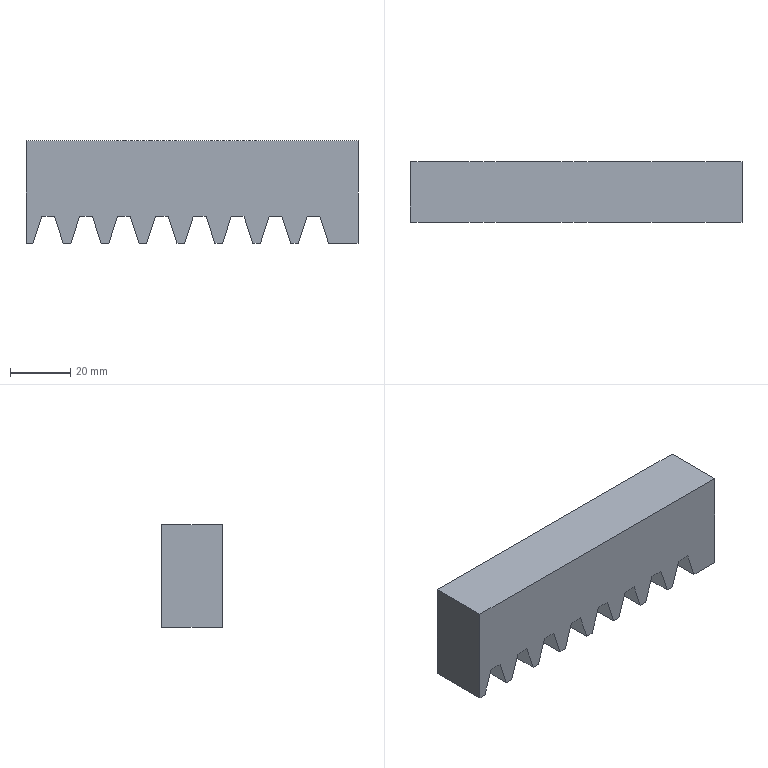Part | SolidWorks | features BaseBody 1 | 1 solid | 46 faces | box 110 x 20 x 34 mm | volume 64536 mm3 | plane 30 | cylinder 16 | commonest cylinder face diameters 94.224 x16
STEP:
#1=CARTESIAN_POINT('',(107.487,369.5,-21.002));
#2=VERTEX_POINT('',#1);
#3=CARTESIAN_POINT('',(109.612,369.5,-21.05));
#4=VERTEX_POINT('',#3);
#5=CARTESIAN_POINT('',(107.487,369.5,-68.114));
#6=DIRECTION('',(0.,1.,0.));
#7=DIRECTION('',(0.,0.,1.));
#8=AXIS2_PLACEMENT_3D('',#5,#6,#7);
#9=CIRCLE('',#8,47.112);
#10=EDGE_CURVE('',#2,#4,#9,.T.);
#11=ORIENTED_EDGE('',*,*,#10,.F.);
#12=CARTESIAN_POINT('',(107.487,389.5,-21.002));
#13=VERTEX_POINT('',#12);
#14=CARTESIAN_POINT('',(107.487,379.5,-21.002));
#15=DIRECTION('',(0.,1.,0.));
#16=VECTOR('',#15,1000.);
#17=LINE('',#14,#16);
#18=EDGE_CURVE('',#2,#13,#17,.T.);
#19=ORIENTED_EDGE('',*,*,#18,.T.);
#20=CARTESIAN_POINT('',(109.612,389.5,-21.05));
#21=VERTEX_POINT('',#20);
#22=CARTESIAN_POINT('',(107.487,389.5,-68.114));
#23=DIRECTION('',(0.,-1.,0.));
#24=DIRECTION('',(0.,0.,1.));
#25=AXIS2_PLACEMENT_3D('',#22,#23,#24);
#26=CIRCLE('',#25,47.112);
#27=EDGE_CURVE('',#21,#13,#26,.T.);
#28=ORIENTED_EDGE('',*,*,#27,.F.);
#29=CARTESIAN_POINT('',(109.612,369.5,-21.05));
#30=DIRECTION('',(0.,1.,0.));
#31=VECTOR('',#30,1000.);
#32=LINE('',#29,#31);
#33=EDGE_CURVE('',#4,#21,#32,.T.);
#34=ORIENTED_EDGE('',*,*,#33,.F.);
#35=EDGE_LOOP('',(#11,#19,#28,#34));
#36=FACE_OUTER_BOUND('',#35,.T.);
#37=CARTESIAN_POINT('',(107.487,379.5,-68.114));
#38=DIRECTION('',(0.,1.,0.));
#39=DIRECTION('',(0.,0.,1.));
#40=AXIS2_PLACEMENT_3D('',#37,#38,#39);
#41=CYLINDRICAL_SURFACE('',#40,47.112);
#42=ADVANCED_FACE('',(#36),#41,.F.);
#43=CARTESIAN_POINT('',(94.927,369.5,-21.002));
#44=VERTEX_POINT('',#43);
#45=CARTESIAN_POINT('',(97.052,369.5,-21.05));
#46=VERTEX_POINT('',#45);
#47=CARTESIAN_POINT('',(94.927,369.5,-68.114));
#48=DIRECTION('',(0.,1.,0.));
#49=DIRECTION('',(0.,0.,1.));
#50=AXIS2_PLACEMENT_3D('',#47,#48,#49);
#51=CIRCLE('',#50,47.112);
#52=EDGE_CURVE('',#44,#46,#51,.T.);
#53=ORIENTED_EDGE('',*,*,#52,.F.);
#54=CARTESIAN_POINT('',(94.927,389.5,-21.002));
#55=VERTEX_POINT('',#54);
#56=CARTESIAN_POINT('',(94.927,379.5,-21.002));
#57=DIRECTION('',(0.,1.,0.));
#58=VECTOR('',#57,1000.);
#59=LINE('',#56,#58);
#60=EDGE_CURVE('',#44,#55,#59,.T.);
#61=ORIENTED_EDGE('',*,*,#60,.T.);
#62=CARTESIAN_POINT('',(97.052,389.5,-21.05));
#63=VERTEX_POINT('',#62);
#64=CARTESIAN_POINT('',(94.927,389.5,-68.114));
#65=DIRECTION('',(0.,-1.,0.));
#66=DIRECTION('',(0.,0.,1.));
#67=AXIS2_PLACEMENT_3D('',#64,#65,#66);
#68=CIRCLE('',#67,47.112);
#69=EDGE_CURVE('',#63,#55,#68,.T.);
#70=ORIENTED_EDGE('',*,*,#69,.F.);
#71=CARTESIAN_POINT('',(97.052,369.5,-21.05));
#72=DIRECTION('',(0.,1.,0.));
#73=VECTOR('',#72,1000.);
#74=LINE('',#71,#73);
#75=EDGE_CURVE('',#46,#63,#74,.T.);
#76=ORIENTED_EDGE('',*,*,#75,.F.);
#77=EDGE_LOOP('',(#53,#61,#70,#76));
#78=FACE_OUTER_BOUND('',#77,.T.);
#79=CARTESIAN_POINT('',(94.927,379.5,-68.114));
#80=DIRECTION('',(0.,1.,0.));
#81=DIRECTION('',(0.,0.,1.));
#82=AXIS2_PLACEMENT_3D('',#79,#80,#81);
#83=CYLINDRICAL_SURFACE('',#82,47.112);
#84=ADVANCED_FACE('',(#78),#83,.F.);
#85=CARTESIAN_POINT('',(82.367,369.5,-21.002));
#86=VERTEX_POINT('',#85);
#87=CARTESIAN_POINT('',(84.492,369.5,-21.05));
#88=VERTEX_POINT('',#87);
#89=CARTESIAN_POINT('',(82.367,369.5,-68.114));
#90=DIRECTION('',(0.,1.,0.));
#91=DIRECTION('',(0.,0.,1.));
#92=AXIS2_PLACEMENT_3D('',#89,#90,#91);
#93=CIRCLE('',#92,47.112);
#94=EDGE_CURVE('',#86,#88,#93,.T.);
#95=ORIENTED_EDGE('',*,*,#94,.F.);
#96=CARTESIAN_POINT('',(82.367,389.5,-21.002));
#97=VERTEX_POINT('',#96);
#98=CARTESIAN_POINT('',(82.367,379.5,-21.002));
#99=DIRECTION('',(0.,1.,0.));
#100=VECTOR('',#99,1000.);
#101=LINE('',#98,#100);
#102=EDGE_CURVE('',#86,#97,#101,.T.);
#103=ORIENTED_EDGE('',*,*,#102,.T.);
#104=CARTESIAN_POINT('',(84.492,389.5,-21.05));
#105=VERTEX_POINT('',#104);
#106=CARTESIAN_POINT('',(82.367,389.5,-68.114));
#107=DIRECTION('',(0.,-1.,0.));
#108=DIRECTION('',(0.,0.,1.));
#109=AXIS2_PLACEMENT_3D('',#106,#107,#108);
#110=CIRCLE('',#109,47.112);
#111=EDGE_CURVE('',#105,#97,#110,.T.);
#112=ORIENTED_EDGE('',*,*,#111,.F.);
#113=CARTESIAN_POINT('',(84.492,369.5,-21.05));
#114=DIRECTION('',(0.,1.,0.));
#115=VECTOR('',#114,1000.);
#116=LINE('',#113,#115);
#117=EDGE_CURVE('',#88,#105,#116,.T.);
#118=ORIENTED_EDGE('',*,*,#117,.F.);
#119=EDGE_LOOP('',(#95,#103,#112,#118));
#120=FACE_OUTER_BOUND('',#119,.T.);
#121=CARTESIAN_POINT('',(82.367,379.5,-68.114));
#122=DIRECTION('',(0.,1.,0.));
#123=DIRECTION('',(0.,0.,1.));
#124=AXIS2_PLACEMENT_3D('',#121,#122,#123);
#125=CYLINDRICAL_SURFACE('',#124,47.112);
#126=ADVANCED_FACE('',(#120),#125,.F.);
#127=CARTESIAN_POINT('',(69.807,369.5,-21.002));
#128=VERTEX_POINT('',#127);
#129=CARTESIAN_POINT('',(71.932,369.5,-21.05));
#130=VERTEX_POINT('',#129);
#131=CARTESIAN_POINT('',(69.807,369.5,-68.114));
#132=DIRECTION('',(0.,1.,0.));
#133=DIRECTION('',(0.,0.,1.));
#134=AXIS2_PLACEMENT_3D('',#131,#132,#133);
#135=CIRCLE('',#134,47.112);
#136=EDGE_CURVE('',#128,#130,#135,.T.);
#137=ORIENTED_EDGE('',*,*,#136,.F.);
#138=CARTESIAN_POINT('',(69.807,389.5,-21.002));
#139=VERTEX_POINT('',#138);
#140=CARTESIAN_POINT('',(69.807,379.5,-21.002));
#141=DIRECTION('',(0.,1.,0.));
#142=VECTOR('',#141,1000.);
#143=LINE('',#140,#142);
#144=EDGE_CURVE('',#128,#139,#143,.T.);
#145=ORIENTED_EDGE('',*,*,#144,.T.);
#146=CARTESIAN_POINT('',(71.932,389.5,-21.05));
#147=VERTEX_POINT('',#146);
#148=CARTESIAN_POINT('',(69.807,389.5,-68.114));
#149=DIRECTION('',(0.,-1.,0.));
#150=DIRECTION('',(0.,0.,1.));
#151=AXIS2_PLACEMENT_3D('',#148,#149,#150);
#152=CIRCLE('',#151,47.112);
#153=EDGE_CURVE('',#147,#139,#152,.T.);
#154=ORIENTED_EDGE('',*,*,#153,.F.);
#155=CARTESIAN_POINT('',(71.932,369.5,-21.05));
#156=DIRECTION('',(0.,1.,0.));
#157=VECTOR('',#156,1000.);
#158=LINE('',#155,#157);
#159=EDGE_CURVE('',#130,#147,#158,.T.);
#160=ORIENTED_EDGE('',*,*,#159,.F.);
#161=EDGE_LOOP('',(#137,#145,#154,#160));
#162=FACE_OUTER_BOUND('',#161,.T.);
#163=CARTESIAN_POINT('',(69.807,379.5,-68.114));
#164=DIRECTION('',(0.,1.,0.));
#165=DIRECTION('',(0.,0.,1.));
#166=AXIS2_PLACEMENT_3D('',#163,#164,#165);
#167=CYLINDRICAL_SURFACE('',#166,47.112);
#168=ADVANCED_FACE('',(#162),#167,.F.);
#169=CARTESIAN_POINT('',(57.247,369.5,-21.002));
#170=VERTEX_POINT('',#169);
#171=CARTESIAN_POINT('',(59.372,369.5,-21.05));
#172=VERTEX_POINT('',#171);
#173=CARTESIAN_POINT('',(57.247,369.5,-68.114));
#174=DIRECTION('',(0.,1.,0.));
#175=DIRECTION('',(0.,0.,1.));
#176=AXIS2_PLACEMENT_3D('',#173,#174,#175);
#177=CIRCLE('',#176,47.112);
#178=EDGE_CURVE('',#170,#172,#177,.T.);
#179=ORIENTED_EDGE('',*,*,#178,.F.);
#180=CARTESIAN_POINT('',(57.247,389.5,-21.002));
#181=VERTEX_POINT('',#180);
#182=CARTESIAN_POINT('',(57.247,379.5,-21.002));
#183=DIRECTION('',(0.,1.,0.));
#184=VECTOR('',#183,1000.);
#185=LINE('',#182,#184);
#186=EDGE_CURVE('',#170,#181,#185,.T.);
#187=ORIENTED_EDGE('',*,*,#186,.T.);
#188=CARTESIAN_POINT('',(59.372,389.5,-21.05));
#189=VERTEX_POINT('',#188);
#190=CARTESIAN_POINT('',(57.247,389.5,-68.114));
#191=DIRECTION('',(0.,-1.,0.));
#192=DIRECTION('',(0.,0.,1.));
#193=AXIS2_PLACEMENT_3D('',#190,#191,#192);
#194=CIRCLE('',#193,47.112);
#195=EDGE_CURVE('',#189,#181,#194,.T.);
#196=ORIENTED_EDGE('',*,*,#195,.F.);
#197=CARTESIAN_POINT('',(59.372,369.5,-21.05));
#198=DIRECTION('',(0.,1.,0.));
#199=VECTOR('',#198,1000.);
#200=LINE('',#197,#199);
#201=EDGE_CURVE('',#172,#189,#200,.T.);
#202=ORIENTED_EDGE('',*,*,#201,.F.);
#203=EDGE_LOOP('',(#179,#187,#196,#202));
#204=FACE_OUTER_BOUND('',#203,.T.);
#205=CARTESIAN_POINT('',(57.247,379.5,-68.114));
#206=DIRECTION('',(0.,1.,0.));
#207=DIRECTION('',(0.,0.,1.));
#208=AXIS2_PLACEMENT_3D('',#205,#206,#207);
#209=CYLINDRICAL_SURFACE('',#208,47.112);
#210=ADVANCED_FACE('',(#204),#209,.F.);
#211=CARTESIAN_POINT('',(44.687,369.5,-21.002));
#212=VERTEX_POINT('',#211);
#213=CARTESIAN_POINT('',(46.812,369.5,-21.05));
#214=VERTEX_POINT('',#213);
#215=CARTESIAN_POINT('',(44.687,369.5,-68.114));
#216=DIRECTION('',(0.,1.,0.));
#217=DIRECTION('',(0.,0.,1.));
#218=AXIS2_PLACEMENT_3D('',#215,#216,#217);
#219=CIRCLE('',#218,47.112);
#220=EDGE_CURVE('',#212,#214,#219,.T.);
#221=ORIENTED_EDGE('',*,*,#220,.F.);
#222=CARTESIAN_POINT('',(44.687,389.5,-21.002));
#223=VERTEX_POINT('',#222);
#224=CARTESIAN_POINT('',(44.687,379.5,-21.002));
#225=DIRECTION('',(0.,1.,0.));
#226=VECTOR('',#225,1000.);
#227=LINE('',#224,#226);
#228=EDGE_CURVE('',#212,#223,#227,.T.);
#229=ORIENTED_EDGE('',*,*,#228,.T.);
#230=CARTESIAN_POINT('',(46.812,389.5,-21.05));
#231=VERTEX_POINT('',#230);
#232=CARTESIAN_POINT('',(44.687,389.5,-68.114));
#233=DIRECTION('',(0.,-1.,0.));
#234=DIRECTION('',(0.,0.,1.));
#235=AXIS2_PLACEMENT_3D('',#232,#233,#234);
#236=CIRCLE('',#235,47.112);
#237=EDGE_CURVE('',#231,#223,#236,.T.);
#238=ORIENTED_EDGE('',*,*,#237,.F.);
#239=CARTESIAN_POINT('',(46.812,369.5,-21.05));
#240=DIRECTION('',(0.,1.,0.));
#241=VECTOR('',#240,1000.);
#242=LINE('',#239,#241);
#243=EDGE_CURVE('',#214,#231,#242,.T.);
#244=ORIENTED_EDGE('',*,*,#243,.F.);
#245=EDGE_LOOP('',(#221,#229,#238,#244));
#246=FACE_OUTER_BOUND('',#245,.T.);
#247=CARTESIAN_POINT('',(44.687,379.5,-68.114));
#248=DIRECTION('',(0.,1.,0.));
#249=DIRECTION('',(0.,0.,1.));
#250=AXIS2_PLACEMENT_3D('',#247,#248,#249);
#251=CYLINDRICAL_SURFACE('',#250,47.112);
#252=ADVANCED_FACE('',(#246),#251,.F.);
#253=CARTESIAN_POINT('',(32.127,369.5,-21.002));
#254=VERTEX_POINT('',#253);
#255=CARTESIAN_POINT('',(34.252,369.5,-21.05));
#256=VERTEX_POINT('',#255);
#257=CARTESIAN_POINT('',(32.127,369.5,-68.114));
#258=DIRECTION('',(0.,1.,0.));
#259=DIRECTION('',(0.,0.,1.));
#260=AXIS2_PLACEMENT_3D('',#257,#258,#259);
#261=CIRCLE('',#260,47.112);
#262=EDGE_CURVE('',#254,#256,#261,.T.);
#263=ORIENTED_EDGE('',*,*,#262,.F.);
#264=CARTESIAN_POINT('',(32.127,389.5,-21.002));
#265=VERTEX_POINT('',#264);
#266=CARTESIAN_POINT('',(32.127,379.5,-21.002));
#267=DIRECTION('',(0.,1.,0.));
#268=VECTOR('',#267,1000.);
#269=LINE('',#266,#268);
#270=EDGE_CURVE('',#254,#265,#269,.T.);
#271=ORIENTED_EDGE('',*,*,#270,.T.);
#272=CARTESIAN_POINT('',(34.252,389.5,-21.05));
#273=VERTEX_POINT('',#272);
#274=CARTESIAN_POINT('',(32.127,389.5,-68.114));
#275=DIRECTION('',(0.,-1.,0.));
#276=DIRECTION('',(0.,0.,1.));
#277=AXIS2_PLACEMENT_3D('',#274,#275,#276);
#278=CIRCLE('',#277,47.112);
#279=EDGE_CURVE('',#273,#265,#278,.T.);
#280=ORIENTED_EDGE('',*,*,#279,.F.);
#281=CARTESIAN_POINT('',(34.252,369.5,-21.05));
#282=DIRECTION('',(0.,1.,0.));
#283=VECTOR('',#282,1000.);
#284=LINE('',#281,#283);
#285=EDGE_CURVE('',#256,#273,#284,.T.);
#286=ORIENTED_EDGE('',*,*,#285,.F.);
#287=EDGE_LOOP('',(#263,#271,#280,#286));
#288=FACE_OUTER_BOUND('',#287,.T.);
#289=CARTESIAN_POINT('',(32.127,379.5,-68.114));
#290=DIRECTION('',(0.,1.,0.));
#291=DIRECTION('',(0.,0.,1.));
#292=AXIS2_PLACEMENT_3D('',#289,#290,#291);
#293=CYLINDRICAL_SURFACE('',#292,47.112);
#294=ADVANCED_FACE('',(#288),#293,.F.);
#295=CARTESIAN_POINT('',(19.567,369.5,-21.002));
#296=VERTEX_POINT('',#295);
#297=CARTESIAN_POINT('',(21.692,369.5,-21.05));
#298=VERTEX_POINT('',#297);
#299=CARTESIAN_POINT('',(19.567,369.5,-68.114));
#300=DIRECTION('',(0.,1.,0.));
#301=DIRECTION('',(0.,0.,1.));
#302=AXIS2_PLACEMENT_3D('',#299,#300,#301);
#303=CIRCLE('',#302,47.112);
#304=EDGE_CURVE('',#296,#298,#303,.T.);
#305=ORIENTED_EDGE('',*,*,#304,.F.);
#306=CARTESIAN_POINT('',(19.567,389.5,-21.002));
#307=VERTEX_POINT('',#306);
#308=CARTESIAN_POINT('',(19.567,379.5,-21.002));
#309=DIRECTION('',(0.,1.,0.));
#310=VECTOR('',#309,1000.);
#311=LINE('',#308,#310);
#312=EDGE_CURVE('',#296,#307,#311,.T.);
#313=ORIENTED_EDGE('',*,*,#312,.T.);
#314=CARTESIAN_POINT('',(21.692,389.5,-21.05));
#315=VERTEX_POINT('',#314);
#316=CARTESIAN_POINT('',(19.567,389.5,-68.114));
#317=DIRECTION('',(0.,-1.,0.));
#318=DIRECTION('',(0.,0.,1.));
#319=AXIS2_PLACEMENT_3D('',#316,#317,#318);
#320=CIRCLE('',#319,47.112);
#321=EDGE_CURVE('',#315,#307,#320,.T.);
#322=ORIENTED_EDGE('',*,*,#321,.F.);
#323=CARTESIAN_POINT('',(21.692,369.5,-21.05));
#324=DIRECTION('',(0.,1.,0.));
#325=VECTOR('',#324,1000.);
#326=LINE('',#323,#325);
#327=EDGE_CURVE('',#298,#315,#326,.T.);
#328=ORIENTED_EDGE('',*,*,#327,.F.);
#329=EDGE_LOOP('',(#305,#313,#322,#328));
#330=FACE_OUTER_BOUND('',#329,.T.);
#331=CARTESIAN_POINT('',(19.567,379.5,-68.114));
#332=DIRECTION('',(0.,1.,0.));
#333=DIRECTION('',(0.,0.,1.));
#334=AXIS2_PLACEMENT_3D('',#331,#332,#333);
#335=CYLINDRICAL_SURFACE('',#334,47.112);
#336=ADVANCED_FACE('',(#330),#335,.F.);
#337=CARTESIAN_POINT('',(112.513,369.5,-30.));
#338=VERTEX_POINT('',#337);
#339=CARTESIAN_POINT('',(109.612,369.5,-21.05));
#340=DIRECTION('',(0.3083,0.,-0.9513));
#341=VECTOR('',#340,1000.);
#342=LINE('',#339,#341);
#343=EDGE_CURVE('',#4,#338,#342,.T.);
#344=ORIENTED_EDGE('',*,*,#343,.T.);
#345=CARTESIAN_POINT('',(122.247,369.5,-30.));
#346=VERTEX_POINT('',#345);
#347=CARTESIAN_POINT('',(77.247,369.5,-30.));
#348=DIRECTION('',(1.,0.,0.));
#349=VECTOR('',#348,1000.);
#350=LINE('',#347,#349);
#351=EDGE_CURVE('',#338,#346,#350,.T.);
#352=ORIENTED_EDGE('',*,*,#351,.T.);
#353=CARTESIAN_POINT('',(122.247,369.5,4.));
#354=VERTEX_POINT('',#353);
#355=CARTESIAN_POINT('',(122.247,369.5,-76.043));
#356=DIRECTION('',(0.,0.,1.));
#357=VECTOR('',#356,1000.);
#358=LINE('',#355,#357);
#359=EDGE_CURVE('',#346,#354,#358,.T.);
#360=ORIENTED_EDGE('',*,*,#359,.T.);
#361=CARTESIAN_POINT('',(12.247,369.5,4.));
#362=VERTEX_POINT('',#361);
#363=CARTESIAN_POINT('',(77.247,369.5,4.));
#364=DIRECTION('',(-1.,0.,0.));
#365=VECTOR('',#364,1000.);
#366=LINE('',#363,#365);
#367=EDGE_CURVE('',#354,#362,#366,.T.);
#368=ORIENTED_EDGE('',*,*,#367,.T.);
#369=CARTESIAN_POINT('',(12.247,369.5,-30.));
#370=VERTEX_POINT('',#369);
#371=CARTESIAN_POINT('',(12.247,369.5,-76.043));
#372=DIRECTION('',(0.,0.,-1.));
#373=VECTOR('',#372,1000.);
#374=LINE('',#371,#373);
#375=EDGE_CURVE('',#362,#370,#374,.T.);
#376=ORIENTED_EDGE('',*,*,#375,.T.);
#377=CARTESIAN_POINT('',(14.54,369.5,-30.));
#378=VERTEX_POINT('',#377);
#379=CARTESIAN_POINT('',(77.247,369.5,-30.));
#380=DIRECTION('',(1.,0.,0.));
#381=VECTOR('',#380,1000.);
#382=LINE('',#379,#381);
#383=EDGE_CURVE('',#370,#378,#382,.T.);
#384=ORIENTED_EDGE('',*,*,#383,.T.);
#385=CARTESIAN_POINT('',(17.441,369.5,-21.05));
#386=VERTEX_POINT('',#385);
#387=CARTESIAN_POINT('',(14.54,369.5,-30.));
#388=DIRECTION('',(0.3083,0.,0.9513));
#389=VECTOR('',#388,1000.);
#390=LINE('',#387,#389);
#391=EDGE_CURVE('',#378,#386,#390,.T.);
#392=ORIENTED_EDGE('',*,*,#391,.T.);
#393=CARTESIAN_POINT('',(19.567,369.5,-68.114));
#394=DIRECTION('',(0.,1.,0.));
#395=DIRECTION('',(0.,0.,1.));
#396=AXIS2_PLACEMENT_3D('',#393,#394,#395);
#397=CIRCLE('',#396,47.112);
#398=EDGE_CURVE('',#386,#296,#397,.T.);
#399=ORIENTED_EDGE('',*,*,#398,.T.);
#400=ORIENTED_EDGE('',*,*,#304,.T.);
#401=CARTESIAN_POINT('',(24.593,369.5,-30.));
#402=VERTEX_POINT('',#401);
#403=CARTESIAN_POINT('',(43.101,369.5,-87.109));
#404=DIRECTION('',(0.3083,0.,-0.9513));
#405=VECTOR('',#404,1000.);
#406=LINE('',#403,#405);
#407=EDGE_CURVE('',#298,#402,#406,.T.);
#408=ORIENTED_EDGE('',*,*,#407,.T.);
#409=CARTESIAN_POINT('',(27.1,369.5,-30.));
#410=VERTEX_POINT('',#409);
#411=CARTESIAN_POINT('',(77.247,369.5,-30.));
#412=DIRECTION('',(1.,0.,0.));
#413=VECTOR('',#412,1000.);
#414=LINE('',#411,#413);
#415=EDGE_CURVE('',#402,#410,#414,.T.);
#416=ORIENTED_EDGE('',*,*,#415,.T.);
#417=CARTESIAN_POINT('',(30.001,369.5,-21.05));
#418=VERTEX_POINT('',#417);
#419=CARTESIAN_POINT('',(27.1,369.5,-30.));
#420=DIRECTION('',(0.3083,0.,0.9513));
#421=VECTOR('',#420,1000.);
#422=LINE('',#419,#421);
#423=EDGE_CURVE('',#410,#418,#422,.T.);
#424=ORIENTED_EDGE('',*,*,#423,.T.);
#425=CARTESIAN_POINT('',(32.127,369.5,-68.114));
#426=DIRECTION('',(0.,1.,0.));
#427=DIRECTION('',(0.,0.,1.));
#428=AXIS2_PLACEMENT_3D('',#425,#426,#427);
#429=CIRCLE('',#428,47.112);
#430=EDGE_CURVE('',#418,#254,#429,.T.);
#431=ORIENTED_EDGE('',*,*,#430,.T.);
#432=ORIENTED_EDGE('',*,*,#262,.T.);
#433=CARTESIAN_POINT('',(37.153,369.5,-30.));
#434=VERTEX_POINT('',#433);
#435=CARTESIAN_POINT('',(34.252,369.5,-21.05));
#436=DIRECTION('',(0.3083,0.,-0.9513));
#437=VECTOR('',#436,1000.);
#438=LINE('',#435,#437);
#439=EDGE_CURVE('',#256,#434,#438,.T.);
#440=ORIENTED_EDGE('',*,*,#439,.T.);
#441=CARTESIAN_POINT('',(39.66,369.5,-30.));
#442=VERTEX_POINT('',#441);
#443=CARTESIAN_POINT('',(77.247,369.5,-30.));
#444=DIRECTION('',(1.,0.,0.));
#445=VECTOR('',#444,1000.);
#446=LINE('',#443,#445);
#447=EDGE_CURVE('',#434,#442,#446,.T.);
#448=ORIENTED_EDGE('',*,*,#447,.T.);
#449=CARTESIAN_POINT('',(42.561,369.5,-21.05));
#450=VERTEX_POINT('',#449);
#451=CARTESIAN_POINT('',(39.66,369.5,-30.));
#452=DIRECTION('',(0.3083,0.,0.9513));
#453=VECTOR('',#452,1000.);
#454=LINE('',#451,#453);
#455=EDGE_CURVE('',#442,#450,#454,.T.);
#456=ORIENTED_EDGE('',*,*,#455,.T.);
#457=CARTESIAN_POINT('',(44.687,369.5,-68.114));
#458=DIRECTION('',(0.,1.,0.));
#459=DIRECTION('',(0.,0.,1.));
#460=AXIS2_PLACEMENT_3D('',#457,#458,#459);
#461=CIRCLE('',#460,47.112);
#462=EDGE_CURVE('',#450,#212,#461,.T.);
#463=ORIENTED_EDGE('',*,*,#462,.T.);
#464=ORIENTED_EDGE('',*,*,#220,.T.);
#465=CARTESIAN_POINT('',(49.713,369.5,-30.));
#466=VERTEX_POINT('',#465);
#467=CARTESIAN_POINT('',(46.812,369.5,-21.05));
#468=DIRECTION('',(0.3083,0.,-0.9513));
#469=VECTOR('',#468,1000.);
#470=LINE('',#467,#469);
#471=EDGE_CURVE('',#214,#466,#470,.T.);
#472=ORIENTED_EDGE('',*,*,#471,.T.);
#473=CARTESIAN_POINT('',(52.22,369.5,-30.));
#474=VERTEX_POINT('',#473);
#475=CARTESIAN_POINT('',(77.247,369.5,-30.));
#476=DIRECTION('',(1.,0.,0.));
#477=VECTOR('',#476,1000.);
#478=LINE('',#475,#477);
#479=EDGE_CURVE('',#466,#474,#478,.T.);
#480=ORIENTED_EDGE('',*,*,#479,.T.);
#481=CARTESIAN_POINT('',(55.121,369.5,-21.05));
#482=VERTEX_POINT('',#481);
#483=CARTESIAN_POINT('',(52.22,369.5,-30.));
#484=DIRECTION('',(0.3083,0.,0.9513));
#485=VECTOR('',#484,1000.);
#486=LINE('',#483,#485);
#487=EDGE_CURVE('',#474,#482,#486,.T.);
#488=ORIENTED_EDGE('',*,*,#487,.T.);
#489=CARTESIAN_POINT('',(57.247,369.5,-68.114));
#490=DIRECTION('',(0.,1.,0.));
#491=DIRECTION('',(0.,0.,1.));
#492=AXIS2_PLACEMENT_3D('',#489,#490,#491);
#493=CIRCLE('',#492,47.112);
#494=EDGE_CURVE('',#482,#170,#493,.T.);
#495=ORIENTED_EDGE('',*,*,#494,.T.);
#496=ORIENTED_EDGE('',*,*,#178,.T.);
#497=CARTESIAN_POINT('',(62.273,369.5,-30.));
#498=VERTEX_POINT('',#497);
#499=CARTESIAN_POINT('',(59.372,369.5,-21.05));
#500=DIRECTION('',(0.3083,0.,-0.9513));
#501=VECTOR('',#500,1000.);
#502=LINE('',#499,#501);
#503=EDGE_CURVE('',#172,#498,#502,.T.);
#504=ORIENTED_EDGE('',*,*,#503,.T.);
#505=CARTESIAN_POINT('',(64.78,369.5,-30.));
#506=VERTEX_POINT('',#505);
#507=CARTESIAN_POINT('',(77.247,369.5,-30.));
#508=DIRECTION('',(1.,0.,0.));
#509=VECTOR('',#508,1000.);
#510=LINE('',#507,#509);
#511=EDGE_CURVE('',#498,#506,#510,.T.);
#512=ORIENTED_EDGE('',*,*,#511,.T.);
#513=CARTESIAN_POINT('',(67.681,369.5,-21.05));
#514=VERTEX_POINT('',#513);
#515=CARTESIAN_POINT('',(64.78,369.5,-30.));
#516=DIRECTION('',(0.3083,0.,0.9513));
#517=VECTOR('',#516,1000.);
#518=LINE('',#515,#517);
#519=EDGE_CURVE('',#506,#514,#518,.T.);
#520=ORIENTED_EDGE('',*,*,#519,.T.);
#521=CARTESIAN_POINT('',(69.807,369.5,-68.114));
#522=DIRECTION('',(0.,1.,0.));
#523=DIRECTION('',(0.,0.,1.));
#524=AXIS2_PLACEMENT_3D('',#521,#522,#523);
#525=CIRCLE('',#524,47.112);
#526=EDGE_CURVE('',#514,#128,#525,.T.);
#527=ORIENTED_EDGE('',*,*,#526,.T.);
#528=ORIENTED_EDGE('',*,*,#136,.T.);
#529=CARTESIAN_POINT('',(74.833,369.5,-30.));
#530=VERTEX_POINT('',#529);
#531=CARTESIAN_POINT('',(71.932,369.5,-21.05));
#532=DIRECTION('',(0.3083,0.,-0.9513));
#533=VECTOR('',#532,1000.);
#534=LINE('',#531,#533);
#535=EDGE_CURVE('',#130,#530,#534,.T.);
#536=ORIENTED_EDGE('',*,*,#535,.T.);
#537=CARTESIAN_POINT('',(77.34,369.5,-30.));
#538=VERTEX_POINT('',#537);
#539=CARTESIAN_POINT('',(77.247,369.5,-30.));
#540=DIRECTION('',(1.,0.,0.));
#541=VECTOR('',#540,1000.);
#542=LINE('',#539,#541);
#543=EDGE_CURVE('',#530,#538,#542,.T.);
#544=ORIENTED_EDGE('',*,*,#543,.T.);
#545=CARTESIAN_POINT('',(80.241,369.5,-21.05));
#546=VERTEX_POINT('',#545);
#547=CARTESIAN_POINT('',(77.34,369.5,-30.));
#548=DIRECTION('',(0.3083,0.,0.9513));
#549=VECTOR('',#548,1000.);
#550=LINE('',#547,#549);
#551=EDGE_CURVE('',#538,#546,#550,.T.);
#552=ORIENTED_EDGE('',*,*,#551,.T.);
#553=CARTESIAN_POINT('',(82.367,369.5,-68.114));
#554=DIRECTION('',(0.,1.,0.));
#555=DIRECTION('',(0.,0.,1.));
#556=AXIS2_PLACEMENT_3D('',#553,#554,#555);
#557=CIRCLE('',#556,47.112);
#558=EDGE_CURVE('',#546,#86,#557,.T.);
#559=ORIENTED_EDGE('',*,*,#558,.T.);
#560=ORIENTED_EDGE('',*,*,#94,.T.);
#561=CARTESIAN_POINT('',(87.393,369.5,-30.));
#562=VERTEX_POINT('',#561);
#563=CARTESIAN_POINT('',(84.492,369.5,-21.05));
#564=DIRECTION('',(0.3083,0.,-0.9513));
#565=VECTOR('',#564,1000.);
#566=LINE('',#563,#565);
#567=EDGE_CURVE('',#88,#562,#566,.T.);
#568=ORIENTED_EDGE('',*,*,#567,.T.);
#569=CARTESIAN_POINT('',(89.9,369.5,-30.));
#570=VERTEX_POINT('',#569);
#571=CARTESIAN_POINT('',(77.247,369.5,-30.));
#572=DIRECTION('',(1.,0.,0.));
#573=VECTOR('',#572,1000.);
#574=LINE('',#571,#573);
#575=EDGE_CURVE('',#562,#570,#574,.T.);
#576=ORIENTED_EDGE('',*,*,#575,.T.);
#577=CARTESIAN_POINT('',(92.801,369.5,-21.05));
#578=VERTEX_POINT('',#577);
#579=CARTESIAN_POINT('',(89.9,369.5,-30.));
#580=DIRECTION('',(0.3083,0.,0.9513));
#581=VECTOR('',#580,1000.);
#582=LINE('',#579,#581);
#583=EDGE_CURVE('',#570,#578,#582,.T.);
#584=ORIENTED_EDGE('',*,*,#583,.T.);
#585=CARTESIAN_POINT('',(94.927,369.5,-68.114));
#586=DIRECTION('',(0.,1.,0.));
#587=DIRECTION('',(0.,0.,1.));
#588=AXIS2_PLACEMENT_3D('',#585,#586,#587);
#589=CIRCLE('',#588,47.112);
#590=EDGE_CURVE('',#578,#44,#589,.T.);
#591=ORIENTED_EDGE('',*,*,#590,.T.);
#592=ORIENTED_EDGE('',*,*,#52,.T.);
#593=CARTESIAN_POINT('',(99.953,369.5,-30.));
#594=VERTEX_POINT('',#593);
#595=CARTESIAN_POINT('',(97.052,369.5,-21.05));
#596=DIRECTION('',(0.3083,0.,-0.9513));
#597=VECTOR('',#596,1000.);
#598=LINE('',#595,#597);
#599=EDGE_CURVE('',#46,#594,#598,.T.);
#600=ORIENTED_EDGE('',*,*,#599,.T.);
#601=CARTESIAN_POINT('',(102.46,369.5,-30.));
#602=VERTEX_POINT('',#601);
#603=CARTESIAN_POINT('',(77.247,369.5,-30.));
#604=DIRECTION('',(1.,0.,0.));
#605=VECTOR('',#604,1000.);
#606=LINE('',#603,#605);
#607=EDGE_CURVE('',#594,#602,#606,.T.);
#608=ORIENTED_EDGE('',*,*,#607,.T.);
#609=CARTESIAN_POINT('',(105.361,369.5,-21.05));
#610=VERTEX_POINT('',#609);
#611=CARTESIAN_POINT('',(102.46,369.5,-30.));
#612=DIRECTION('',(0.3083,0.,0.9513));
#613=VECTOR('',#612,1000.);
#614=LINE('',#611,#613);
#615=EDGE_CURVE('',#602,#610,#614,.T.);
#616=ORIENTED_EDGE('',*,*,#615,.T.);
#617=CARTESIAN_POINT('',(107.487,369.5,-68.114));
#618=DIRECTION('',(0.,1.,0.));
#619=DIRECTION('',(0.,0.,1.));
#620=AXIS2_PLACEMENT_3D('',#617,#618,#619);
#621=CIRCLE('',#620,47.112);
#622=EDGE_CURVE('',#610,#2,#621,.T.);
#623=ORIENTED_EDGE('',*,*,#622,.T.);
#624=ORIENTED_EDGE('',*,*,#10,.T.);
#625=EDGE_LOOP('',(#344,#352,#360,#368,#376,#384,#392,#399,#400,#408,#416,#424,#431,#432,#440,#448,#456,#463,#464,#472,#480,#488,#495,#496,#504,#512,#520,#527,#528,#536,#544,#552,#559,#560,#568,#576,#584,#591,#592,#600,#608,#616,#623,#624));
#626=FACE_OUTER_BOUND('',#625,.T.);
#627=CARTESIAN_POINT('',(77.247,369.5,-76.043));
#628=DIRECTION('',(0.,-1.,0.));
#629=DIRECTION('',(0.,0.,-1.));
#630=AXIS2_PLACEMENT_3D('',#627,#628,#629);
#631=PLANE('',#630);
#632=ADVANCED_FACE('',(#626),#631,.T.);
#633=ORIENTED_EDGE('',*,*,#351,.F.);
#634=CARTESIAN_POINT('',(112.513,389.5,-30.));
#635=VERTEX_POINT('',#634);
#636=CARTESIAN_POINT('',(112.513,389.115,-30.));
#637=DIRECTION('',(0.,-1.,0.));
#638=VECTOR('',#637,1000.);
#639=LINE('',#636,#638);
#640=EDGE_CURVE('',#635,#338,#639,.T.);
#641=ORIENTED_EDGE('',*,*,#640,.F.);
#642=CARTESIAN_POINT('',(122.247,389.5,-30.));
#643=VERTEX_POINT('',#642);
#644=CARTESIAN_POINT('',(131.477,389.5,-30.));
#645=DIRECTION('',(-1.,0.,0.));
#646=VECTOR('',#645,1000.);
#647=LINE('',#644,#646);
#648=EDGE_CURVE('',#643,#635,#647,.T.);
#649=ORIENTED_EDGE('',*,*,#648,.F.);
#650=CARTESIAN_POINT('',(122.247,389.115,-30.));
#651=DIRECTION('',(0.,1.,0.));
#652=VECTOR('',#651,1000.);
#653=LINE('',#650,#652);
#654=EDGE_CURVE('',#346,#643,#653,.T.);
#655=ORIENTED_EDGE('',*,*,#654,.F.);
#656=EDGE_LOOP('',(#633,#641,#649,#655));
#657=FACE_OUTER_BOUND('',#656,.T.);
#658=CARTESIAN_POINT('',(131.477,389.115,-30.));
#659=DIRECTION('',(0.,0.,1.));
#660=DIRECTION('',(1.,0.,0.));
#661=AXIS2_PLACEMENT_3D('',#658,#659,#660);
#662=PLANE('',#661);
#663=ADVANCED_FACE('',(#657),#662,.F.);
#664=ORIENTED_EDGE('',*,*,#33,.T.);
#665=CARTESIAN_POINT('',(111.946,389.5,-28.252));
#666=DIRECTION('',(0.3083,0.,-0.9513));
#667=VECTOR('',#666,1000.);
#668=LINE('',#665,#667);
#669=EDGE_CURVE('',#21,#635,#668,.T.);
#670=ORIENTED_EDGE('',*,*,#669,.T.);
#671=ORIENTED_EDGE('',*,*,#640,.T.);
#672=ORIENTED_EDGE('',*,*,#343,.F.);
#673=EDGE_LOOP('',(#664,#670,#671,#672));
#674=FACE_OUTER_BOUND('',#673,.T.);
#675=CARTESIAN_POINT('',(111.946,294.5,-28.252));
#676=DIRECTION('',(-0.9513,0.,-0.3083));
#677=DIRECTION('',(-0.3083,0.,0.9513));
#678=AXIS2_PLACEMENT_3D('',#675,#676,#677);
#679=PLANE('',#678);
#680=ADVANCED_FACE('',(#674),#679,.T.);
#681=ORIENTED_EDGE('',*,*,#18,.F.);
#682=ORIENTED_EDGE('',*,*,#622,.F.);
#683=CARTESIAN_POINT('',(105.361,389.5,-21.05));
#684=VERTEX_POINT('',#683);
#685=CARTESIAN_POINT('',(105.361,389.5,-21.05));
#686=DIRECTION('',(0.,-1.,0.));
#687=VECTOR('',#686,1000.);
#688=LINE('',#685,#687);
#689=EDGE_CURVE('',#684,#610,#688,.T.);
#690=ORIENTED_EDGE('',*,*,#689,.F.);
#691=CARTESIAN_POINT('',(107.487,389.5,-68.114));
#692=DIRECTION('',(0.,-1.,0.));
#693=DIRECTION('',(0.,0.,1.));
#694=AXIS2_PLACEMENT_3D('',#691,#692,#693);
#695=CIRCLE('',#694,47.112);
#696=EDGE_CURVE('',#13,#684,#695,.T.);
#697=ORIENTED_EDGE('',*,*,#696,.F.);
#698=EDGE_LOOP('',(#681,#682,#690,#697));
#699=FACE_OUTER_BOUND('',#698,.T.);
#700=CARTESIAN_POINT('',(107.487,379.5,-68.114));
#701=DIRECTION('',(0.,1.,0.));
#702=DIRECTION('',(0.,0.,1.));
#703=AXIS2_PLACEMENT_3D('',#700,#701,#702);
#704=CYLINDRICAL_SURFACE('',#703,47.112);
#705=ADVANCED_FACE('',(#699),#704,.F.);
#706=CARTESIAN_POINT('',(102.46,389.5,-30.));
#707=VERTEX_POINT('',#706);
#708=CARTESIAN_POINT('',(102.46,294.5,-30.));
#709=DIRECTION('',(0.,1.,0.));
#710=VECTOR('',#709,1000.);
#711=LINE('',#708,#710);
#712=EDGE_CURVE('',#602,#707,#711,.T.);
#713=ORIENTED_EDGE('',*,*,#712,.T.);
#714=CARTESIAN_POINT('',(105.146,389.5,-21.714));
#715=DIRECTION('',(0.3083,0.,0.9513));
#716=VECTOR('',#715,1000.);
#717=LINE('',#714,#716);
#718=EDGE_CURVE('',#707,#684,#717,.T.);
#719=ORIENTED_EDGE('',*,*,#718,.T.);
#720=ORIENTED_EDGE('',*,*,#689,.T.);
#721=ORIENTED_EDGE('',*,*,#615,.F.);
#722=EDGE_LOOP('',(#713,#719,#720,#721));
#723=FACE_OUTER_BOUND('',#722,.T.);
#724=CARTESIAN_POINT('',(105.146,294.5,-21.714));
#725=DIRECTION('',(0.9513,0.,-0.3083));
#726=DIRECTION('',(-0.3083,0.,-0.9513));
#727=AXIS2_PLACEMENT_3D('',#724,#725,#726);
#728=PLANE('',#727);
#729=ADVANCED_FACE('',(#723),#728,.T.);
#730=ORIENTED_EDGE('',*,*,#607,.F.);
#731=CARTESIAN_POINT('',(99.953,389.5,-30.));
#732=VERTEX_POINT('',#731);
#733=CARTESIAN_POINT('',(99.953,389.115,-30.));
#734=DIRECTION('',(0.,-1.,0.));
#735=VECTOR('',#734,1000.);
#736=LINE('',#733,#735);
#737=EDGE_CURVE('',#732,#594,#736,.T.);
#738=ORIENTED_EDGE('',*,*,#737,.F.);
#739=CARTESIAN_POINT('',(131.477,389.5,-30.));
#740=DIRECTION('',(-1.,0.,0.));
#741=VECTOR('',#740,1000.);
#742=LINE('',#739,#741);
#743=EDGE_CURVE('',#707,#732,#742,.T.);
#744=ORIENTED_EDGE('',*,*,#743,.F.);
#745=ORIENTED_EDGE('',*,*,#712,.F.);
#746=EDGE_LOOP('',(#730,#738,#744,#745));
#747=FACE_OUTER_BOUND('',#746,.T.);
#748=CARTESIAN_POINT('',(131.477,389.115,-30.));
#749=DIRECTION('',(0.,0.,1.));
#750=DIRECTION('',(1.,0.,0.));
#751=AXIS2_PLACEMENT_3D('',#748,#749,#750);
#752=PLANE('',#751);
#753=ADVANCED_FACE('',(#747),#752,.F.);
#754=ORIENTED_EDGE('',*,*,#75,.T.);
#755=CARTESIAN_POINT('',(99.386,389.5,-28.252));
#756=DIRECTION('',(0.3083,0.,-0.9513));
#757=VECTOR('',#756,1000.);
#758=LINE('',#755,#757);
#759=EDGE_CURVE('',#63,#732,#758,.T.);
#760=ORIENTED_EDGE('',*,*,#759,.T.);
#761=ORIENTED_EDGE('',*,*,#737,.T.);
#762=ORIENTED_EDGE('',*,*,#599,.F.);
#763=EDGE_LOOP('',(#754,#760,#761,#762));
#764=FACE_OUTER_BOUND('',#763,.T.);
#765=CARTESIAN_POINT('',(99.386,294.5,-28.252));
#766=DIRECTION('',(-0.9513,0.,-0.3083));
#767=DIRECTION('',(-0.3083,0.,0.9513));
#768=AXIS2_PLACEMENT_3D('',#765,#766,#767);
#769=PLANE('',#768);
#770=ADVANCED_FACE('',(#764),#769,.T.);
#771=ORIENTED_EDGE('',*,*,#60,.F.);
#772=ORIENTED_EDGE('',*,*,#590,.F.);
#773=CARTESIAN_POINT('',(92.801,389.5,-21.05));
#774=VERTEX_POINT('',#773);
#775=CARTESIAN_POINT('',(92.801,389.5,-21.05));
#776=DIRECTION('',(0.,-1.,0.));
#777=VECTOR('',#776,1000.);
#778=LINE('',#775,#777);
#779=EDGE_CURVE('',#774,#578,#778,.T.);
#780=ORIENTED_EDGE('',*,*,#779,.F.);
#781=CARTESIAN_POINT('',(94.927,389.5,-68.114));
#782=DIRECTION('',(0.,-1.,0.));
#783=DIRECTION('',(0.,0.,1.));
#784=AXIS2_PLACEMENT_3D('',#781,#782,#783);
#785=CIRCLE('',#784,47.112);
#786=EDGE_CURVE('',#55,#774,#785,.T.);
#787=ORIENTED_EDGE('',*,*,#786,.F.);
#788=EDGE_LOOP('',(#771,#772,#780,#787));
#789=FACE_OUTER_BOUND('',#788,.T.);
#790=CARTESIAN_POINT('',(94.927,379.5,-68.114));
#791=DIRECTION('',(0.,1.,0.));
#792=DIRECTION('',(0.,0.,1.));
#793=AXIS2_PLACEMENT_3D('',#790,#791,#792);
#794=CYLINDRICAL_SURFACE('',#793,47.112);
#795=ADVANCED_FACE('',(#789),#794,.F.);
#796=CARTESIAN_POINT('',(89.9,389.5,-30.));
#797=VERTEX_POINT('',#796);
#798=CARTESIAN_POINT('',(89.9,294.5,-30.));
#799=DIRECTION('',(0.,1.,0.));
#800=VECTOR('',#799,1000.);
#801=LINE('',#798,#800);
#802=EDGE_CURVE('',#570,#797,#801,.T.);
#803=ORIENTED_EDGE('',*,*,#802,.T.);
#804=CARTESIAN_POINT('',(92.586,389.5,-21.714));
#805=DIRECTION('',(0.3083,0.,0.9513));
#806=VECTOR('',#805,1000.);
#807=LINE('',#804,#806);
#808=EDGE_CURVE('',#797,#774,#807,.T.);
#809=ORIENTED_EDGE('',*,*,#808,.T.);
#810=ORIENTED_EDGE('',*,*,#779,.T.);
#811=ORIENTED_EDGE('',*,*,#583,.F.);
#812=EDGE_LOOP('',(#803,#809,#810,#811));
#813=FACE_OUTER_BOUND('',#812,.T.);
#814=CARTESIAN_POINT('',(92.586,294.5,-21.714));
#815=DIRECTION('',(0.9513,0.,-0.3083));
#816=DIRECTION('',(-0.3083,0.,-0.9513));
#817=AXIS2_PLACEMENT_3D('',#814,#815,#816);
#818=PLANE('',#817);
#819=ADVANCED_FACE('',(#813),#818,.T.);
#820=ORIENTED_EDGE('',*,*,#575,.F.);
#821=CARTESIAN_POINT('',(87.393,389.5,-30.));
#822=VERTEX_POINT('',#821);
#823=CARTESIAN_POINT('',(87.393,389.115,-30.));
#824=DIRECTION('',(0.,-1.,0.));
#825=VECTOR('',#824,1000.);
#826=LINE('',#823,#825);
#827=EDGE_CURVE('',#822,#562,#826,.T.);
#828=ORIENTED_EDGE('',*,*,#827,.F.);
#829=CARTESIAN_POINT('',(131.477,389.5,-30.));
#830=DIRECTION('',(-1.,0.,0.));
#831=VECTOR('',#830,1000.);
#832=LINE('',#829,#831);
#833=EDGE_CURVE('',#797,#822,#832,.T.);
#834=ORIENTED_EDGE('',*,*,#833,.F.);
#835=ORIENTED_EDGE('',*,*,#802,.F.);
#836=EDGE_LOOP('',(#820,#828,#834,#835));
#837=FACE_OUTER_BOUND('',#836,.T.);
#838=CARTESIAN_POINT('',(131.477,389.115,-30.));
#839=DIRECTION('',(0.,0.,1.));
#840=DIRECTION('',(1.,0.,0.));
#841=AXIS2_PLACEMENT_3D('',#838,#839,#840);
#842=PLANE('',#841);
#843=ADVANCED_FACE('',(#837),#842,.F.);
#844=ORIENTED_EDGE('',*,*,#117,.T.);
#845=CARTESIAN_POINT('',(86.826,389.5,-28.252));
#846=DIRECTION('',(0.3083,0.,-0.9513));
#847=VECTOR('',#846,1000.);
#848=LINE('',#845,#847);
#849=EDGE_CURVE('',#105,#822,#848,.T.);
#850=ORIENTED_EDGE('',*,*,#849,.T.);
#851=ORIENTED_EDGE('',*,*,#827,.T.);
#852=ORIENTED_EDGE('',*,*,#567,.F.);
#853=EDGE_LOOP('',(#844,#850,#851,#852));
#854=FACE_OUTER_BOUND('',#853,.T.);
#855=CARTESIAN_POINT('',(86.826,294.5,-28.252));
#856=DIRECTION('',(-0.9513,0.,-0.3083));
#857=DIRECTION('',(-0.3083,0.,0.9513));
#858=AXIS2_PLACEMENT_3D('',#855,#856,#857);
#859=PLANE('',#858);
#860=ADVANCED_FACE('',(#854),#859,.T.);
#861=ORIENTED_EDGE('',*,*,#102,.F.);
#862=ORIENTED_EDGE('',*,*,#558,.F.);
#863=CARTESIAN_POINT('',(80.241,389.5,-21.05));
#864=VERTEX_POINT('',#863);
#865=CARTESIAN_POINT('',(80.241,389.5,-21.05));
#866=DIRECTION('',(0.,-1.,0.));
#867=VECTOR('',#866,1000.);
#868=LINE('',#865,#867);
#869=EDGE_CURVE('',#864,#546,#868,.T.);
#870=ORIENTED_EDGE('',*,*,#869,.F.);
#871=CARTESIAN_POINT('',(82.367,389.5,-68.114));
#872=DIRECTION('',(0.,-1.,0.));
#873=DIRECTION('',(0.,0.,1.));
#874=AXIS2_PLACEMENT_3D('',#871,#872,#873);
#875=CIRCLE('',#874,47.112);
#876=EDGE_CURVE('',#97,#864,#875,.T.);
#877=ORIENTED_EDGE('',*,*,#876,.F.);
#878=EDGE_LOOP('',(#861,#862,#870,#877));
#879=FACE_OUTER_BOUND('',#878,.T.);
#880=CARTESIAN_POINT('',(82.367,379.5,-68.114));
#881=DIRECTION('',(0.,1.,0.));
#882=DIRECTION('',(0.,0.,1.));
#883=AXIS2_PLACEMENT_3D('',#880,#881,#882);
#884=CYLINDRICAL_SURFACE('',#883,47.112);
#885=ADVANCED_FACE('',(#879),#884,.F.);
#886=CARTESIAN_POINT('',(77.34,389.5,-30.));
#887=VERTEX_POINT('',#886);
#888=CARTESIAN_POINT('',(77.34,294.5,-30.));
#889=DIRECTION('',(0.,1.,0.));
#890=VECTOR('',#889,1000.);
#891=LINE('',#888,#890);
#892=EDGE_CURVE('',#538,#887,#891,.T.);
#893=ORIENTED_EDGE('',*,*,#892,.T.);
#894=CARTESIAN_POINT('',(80.026,389.5,-21.714));
#895=DIRECTION('',(0.3083,0.,0.9513));
#896=VECTOR('',#895,1000.);
#897=LINE('',#894,#896);
#898=EDGE_CURVE('',#887,#864,#897,.T.);
#899=ORIENTED_EDGE('',*,*,#898,.T.);
#900=ORIENTED_EDGE('',*,*,#869,.T.);
#901=ORIENTED_EDGE('',*,*,#551,.F.);
#902=EDGE_LOOP('',(#893,#899,#900,#901));
#903=FACE_OUTER_BOUND('',#902,.T.);
#904=CARTESIAN_POINT('',(80.026,294.5,-21.714));
#905=DIRECTION('',(0.9513,0.,-0.3083));
#906=DIRECTION('',(-0.3083,0.,-0.9513));
#907=AXIS2_PLACEMENT_3D('',#904,#905,#906);
#908=PLANE('',#907);
#909=ADVANCED_FACE('',(#903),#908,.T.);
#910=ORIENTED_EDGE('',*,*,#543,.F.);
#911=CARTESIAN_POINT('',(74.833,389.5,-30.));
#912=VERTEX_POINT('',#911);
#913=CARTESIAN_POINT('',(74.833,389.115,-30.));
#914=DIRECTION('',(0.,-1.,0.));
#915=VECTOR('',#914,1000.);
#916=LINE('',#913,#915);
#917=EDGE_CURVE('',#912,#530,#916,.T.);
#918=ORIENTED_EDGE('',*,*,#917,.F.);
#919=CARTESIAN_POINT('',(131.477,389.5,-30.));
#920=DIRECTION('',(-1.,0.,0.));
#921=VECTOR('',#920,1000.);
#922=LINE('',#919,#921);
#923=EDGE_CURVE('',#887,#912,#922,.T.);
#924=ORIENTED_EDGE('',*,*,#923,.F.);
#925=ORIENTED_EDGE('',*,*,#892,.F.);
#926=EDGE_LOOP('',(#910,#918,#924,#925));
#927=FACE_OUTER_BOUND('',#926,.T.);
#928=CARTESIAN_POINT('',(131.477,389.115,-30.));
#929=DIRECTION('',(0.,0.,1.));
#930=DIRECTION('',(1.,0.,0.));
#931=AXIS2_PLACEMENT_3D('',#928,#929,#930);
#932=PLANE('',#931);
#933=ADVANCED_FACE('',(#927),#932,.F.);
#934=ORIENTED_EDGE('',*,*,#159,.T.);
#935=CARTESIAN_POINT('',(74.266,389.5,-28.252));
#936=DIRECTION('',(0.3083,0.,-0.9513));
#937=VECTOR('',#936,1000.);
#938=LINE('',#935,#937);
#939=EDGE_CURVE('',#147,#912,#938,.T.);
#940=ORIENTED_EDGE('',*,*,#939,.T.);
#941=ORIENTED_EDGE('',*,*,#917,.T.);
#942=ORIENTED_EDGE('',*,*,#535,.F.);
#943=EDGE_LOOP('',(#934,#940,#941,#942));
#944=FACE_OUTER_BOUND('',#943,.T.);
#945=CARTESIAN_POINT('',(74.266,294.5,-28.252));
#946=DIRECTION('',(-0.9513,0.,-0.3083));
#947=DIRECTION('',(-0.3083,0.,0.9513));
#948=AXIS2_PLACEMENT_3D('',#945,#946,#947);
#949=PLANE('',#948);
#950=ADVANCED_FACE('',(#944),#949,.T.);
#951=ORIENTED_EDGE('',*,*,#144,.F.);
#952=ORIENTED_EDGE('',*,*,#526,.F.);
#953=CARTESIAN_POINT('',(67.681,389.5,-21.05));
#954=VERTEX_POINT('',#953);
#955=CARTESIAN_POINT('',(67.681,389.5,-21.05));
#956=DIRECTION('',(0.,-1.,0.));
#957=VECTOR('',#956,1000.);
#958=LINE('',#955,#957);
#959=EDGE_CURVE('',#954,#514,#958,.T.);
#960=ORIENTED_EDGE('',*,*,#959,.F.);
#961=CARTESIAN_POINT('',(69.807,389.5,-68.114));
#962=DIRECTION('',(0.,-1.,0.));
#963=DIRECTION('',(0.,0.,1.));
#964=AXIS2_PLACEMENT_3D('',#961,#962,#963);
#965=CIRCLE('',#964,47.112);
#966=EDGE_CURVE('',#139,#954,#965,.T.);
#967=ORIENTED_EDGE('',*,*,#966,.F.);
#968=EDGE_LOOP('',(#951,#952,#960,#967));
#969=FACE_OUTER_BOUND('',#968,.T.);
#970=CARTESIAN_POINT('',(69.807,379.5,-68.114));
#971=DIRECTION('',(0.,1.,0.));
#972=DIRECTION('',(0.,0.,1.));
#973=AXIS2_PLACEMENT_3D('',#970,#971,#972);
#974=CYLINDRICAL_SURFACE('',#973,47.112);
#975=ADVANCED_FACE('',(#969),#974,.F.);
#976=CARTESIAN_POINT('',(64.78,389.5,-30.));
#977=VERTEX_POINT('',#976);
#978=CARTESIAN_POINT('',(64.78,294.5,-30.));
#979=DIRECTION('',(0.,1.,0.));
#980=VECTOR('',#979,1000.);
#981=LINE('',#978,#980);
#982=EDGE_CURVE('',#506,#977,#981,.T.);
#983=ORIENTED_EDGE('',*,*,#982,.T.);
#984=CARTESIAN_POINT('',(67.466,389.5,-21.714));
#985=DIRECTION('',(0.3083,0.,0.9513));
#986=VECTOR('',#985,1000.);
#987=LINE('',#984,#986);
#988=EDGE_CURVE('',#977,#954,#987,.T.);
#989=ORIENTED_EDGE('',*,*,#988,.T.);
#990=ORIENTED_EDGE('',*,*,#959,.T.);
#991=ORIENTED_EDGE('',*,*,#519,.F.);
#992=EDGE_LOOP('',(#983,#989,#990,#991));
#993=FACE_OUTER_BOUND('',#992,.T.);
#994=CARTESIAN_POINT('',(67.466,294.5,-21.714));
#995=DIRECTION('',(0.9513,0.,-0.3083));
#996=DIRECTION('',(-0.3083,0.,-0.9513));
#997=AXIS2_PLACEMENT_3D('',#994,#995,#996);
#998=PLANE('',#997);
#999=ADVANCED_FACE('',(#993),#998,.T.);
#1000=ORIENTED_EDGE('',*,*,#511,.F.);
#1001=CARTESIAN_POINT('',(62.273,389.5,-30.));
#1002=VERTEX_POINT('',#1001);
#1003=CARTESIAN_POINT('',(62.273,389.115,-30.));
#1004=DIRECTION('',(0.,-1.,0.));
#1005=VECTOR('',#1004,1000.);
#1006=LINE('',#1003,#1005);
#1007=EDGE_CURVE('',#1002,#498,#1006,.T.);
#1008=ORIENTED_EDGE('',*,*,#1007,.F.);
#1009=CARTESIAN_POINT('',(131.477,389.5,-30.));
#1010=DIRECTION('',(-1.,0.,0.));
#1011=VECTOR('',#1010,1000.);
#1012=LINE('',#1009,#1011);
#1013=EDGE_CURVE('',#977,#1002,#1012,.T.);
#1014=ORIENTED_EDGE('',*,*,#1013,.F.);
#1015=ORIENTED_EDGE('',*,*,#982,.F.);
#1016=EDGE_LOOP('',(#1000,#1008,#1014,#1015));
#1017=FACE_OUTER_BOUND('',#1016,.T.);
#1018=CARTESIAN_POINT('',(131.477,389.115,-30.));
#1019=DIRECTION('',(0.,0.,1.));
#1020=DIRECTION('',(1.,0.,0.));
#1021=AXIS2_PLACEMENT_3D('',#1018,#1019,#1020);
#1022=PLANE('',#1021);
#1023=ADVANCED_FACE('',(#1017),#1022,.F.);
#1024=ORIENTED_EDGE('',*,*,#201,.T.);
#1025=CARTESIAN_POINT('',(61.706,389.5,-28.252));
#1026=DIRECTION('',(0.3083,0.,-0.9513));
#1027=VECTOR('',#1026,1000.);
#1028=LINE('',#1025,#1027);
#1029=EDGE_CURVE('',#189,#1002,#1028,.T.);
#1030=ORIENTED_EDGE('',*,*,#1029,.T.);
#1031=ORIENTED_EDGE('',*,*,#1007,.T.);
#1032=ORIENTED_EDGE('',*,*,#503,.F.);
#1033=EDGE_LOOP('',(#1024,#1030,#1031,#1032));
#1034=FACE_OUTER_BOUND('',#1033,.T.);
#1035=CARTESIAN_POINT('',(61.706,294.5,-28.252));
#1036=DIRECTION('',(-0.9513,0.,-0.3083));
#1037=DIRECTION('',(-0.3083,0.,0.9513));
#1038=AXIS2_PLACEMENT_3D('',#1035,#1036,#1037);
#1039=PLANE('',#1038);
#1040=ADVANCED_FACE('',(#1034),#1039,.T.);
#1041=ORIENTED_EDGE('',*,*,#186,.F.);
#1042=ORIENTED_EDGE('',*,*,#494,.F.);
#1043=CARTESIAN_POINT('',(55.121,389.5,-21.05));
#1044=VERTEX_POINT('',#1043);
#1045=CARTESIAN_POINT('',(55.121,389.5,-21.05));
#1046=DIRECTION('',(0.,-1.,0.));
#1047=VECTOR('',#1046,1000.);
#1048=LINE('',#1045,#1047);
#1049=EDGE_CURVE('',#1044,#482,#1048,.T.);
#1050=ORIENTED_EDGE('',*,*,#1049,.F.);
#1051=CARTESIAN_POINT('',(57.247,389.5,-68.114));
#1052=DIRECTION('',(0.,-1.,0.));
#1053=DIRECTION('',(0.,0.,1.));
#1054=AXIS2_PLACEMENT_3D('',#1051,#1052,#1053);
#1055=CIRCLE('',#1054,47.112);
#1056=EDGE_CURVE('',#181,#1044,#1055,.T.);
#1057=ORIENTED_EDGE('',*,*,#1056,.F.);
#1058=EDGE_LOOP('',(#1041,#1042,#1050,#1057));
#1059=FACE_OUTER_BOUND('',#1058,.T.);
#1060=CARTESIAN_POINT('',(57.247,379.5,-68.114));
#1061=DIRECTION('',(0.,1.,0.));
#1062=DIRECTION('',(0.,0.,1.));
#1063=AXIS2_PLACEMENT_3D('',#1060,#1061,#1062);
#1064=CYLINDRICAL_SURFACE('',#1063,47.112);
#1065=ADVANCED_FACE('',(#1059),#1064,.F.);
#1066=CARTESIAN_POINT('',(52.22,389.5,-30.));
#1067=VERTEX_POINT('',#1066);
#1068=CARTESIAN_POINT('',(52.22,294.5,-30.));
#1069=DIRECTION('',(0.,1.,0.));
#1070=VECTOR('',#1069,1000.);
#1071=LINE('',#1068,#1070);
#1072=EDGE_CURVE('',#474,#1067,#1071,.T.);
#1073=ORIENTED_EDGE('',*,*,#1072,.T.);
#1074=CARTESIAN_POINT('',(54.906,389.5,-21.714));
#1075=DIRECTION('',(0.3083,0.,0.9513));
#1076=VECTOR('',#1075,1000.);
#1077=LINE('',#1074,#1076);
#1078=EDGE_CURVE('',#1067,#1044,#1077,.T.);
#1079=ORIENTED_EDGE('',*,*,#1078,.T.);
#1080=ORIENTED_EDGE('',*,*,#1049,.T.);
#1081=ORIENTED_EDGE('',*,*,#487,.F.);
#1082=EDGE_LOOP('',(#1073,#1079,#1080,#1081));
#1083=FACE_OUTER_BOUND('',#1082,.T.);
#1084=CARTESIAN_POINT('',(54.906,294.5,-21.714));
#1085=DIRECTION('',(0.9513,0.,-0.3083));
#1086=DIRECTION('',(-0.3083,0.,-0.9513));
#1087=AXIS2_PLACEMENT_3D('',#1084,#1085,#1086);
#1088=PLANE('',#1087);
#1089=ADVANCED_FACE('',(#1083),#1088,.T.);
#1090=ORIENTED_EDGE('',*,*,#479,.F.);
#1091=CARTESIAN_POINT('',(49.713,389.5,-30.));
#1092=VERTEX_POINT('',#1091);
#1093=CARTESIAN_POINT('',(49.713,389.115,-30.));
#1094=DIRECTION('',(0.,-1.,0.));
#1095=VECTOR('',#1094,1000.);
#1096=LINE('',#1093,#1095);
#1097=EDGE_CURVE('',#1092,#466,#1096,.T.);
#1098=ORIENTED_EDGE('',*,*,#1097,.F.);
#1099=CARTESIAN_POINT('',(131.477,389.5,-30.));
#1100=DIRECTION('',(-1.,0.,0.));
#1101=VECTOR('',#1100,1000.);
#1102=LINE('',#1099,#1101);
#1103=EDGE_CURVE('',#1067,#1092,#1102,.T.);
#1104=ORIENTED_EDGE('',*,*,#1103,.F.);
#1105=ORIENTED_EDGE('',*,*,#1072,.F.);
#1106=EDGE_LOOP('',(#1090,#1098,#1104,#1105));
#1107=FACE_OUTER_BOUND('',#1106,.T.);
#1108=CARTESIAN_POINT('',(131.477,389.115,-30.));
#1109=DIRECTION('',(0.,0.,1.));
#1110=DIRECTION('',(1.,0.,0.));
#1111=AXIS2_PLACEMENT_3D('',#1108,#1109,#1110);
#1112=PLANE('',#1111);
#1113=ADVANCED_FACE('',(#1107),#1112,.F.);
#1114=ORIENTED_EDGE('',*,*,#243,.T.);
#1115=CARTESIAN_POINT('',(49.146,389.5,-28.252));
#1116=DIRECTION('',(0.3083,0.,-0.9513));
#1117=VECTOR('',#1116,1000.);
#1118=LINE('',#1115,#1117);
#1119=EDGE_CURVE('',#231,#1092,#1118,.T.);
#1120=ORIENTED_EDGE('',*,*,#1119,.T.);
#1121=ORIENTED_EDGE('',*,*,#1097,.T.);
#1122=ORIENTED_EDGE('',*,*,#471,.F.);
#1123=EDGE_LOOP('',(#1114,#1120,#1121,#1122));
#1124=FACE_OUTER_BOUND('',#1123,.T.);
#1125=CARTESIAN_POINT('',(49.146,294.5,-28.252));
#1126=DIRECTION('',(-0.9513,0.,-0.3083));
#1127=DIRECTION('',(-0.3083,0.,0.9513));
#1128=AXIS2_PLACEMENT_3D('',#1125,#1126,#1127);
#1129=PLANE('',#1128);
#1130=ADVANCED_FACE('',(#1124),#1129,.T.);
#1131=ORIENTED_EDGE('',*,*,#228,.F.);
#1132=ORIENTED_EDGE('',*,*,#462,.F.);
#1133=CARTESIAN_POINT('',(42.561,389.5,-21.05));
#1134=VERTEX_POINT('',#1133);
#1135=CARTESIAN_POINT('',(42.561,389.5,-21.05));
#1136=DIRECTION('',(0.,-1.,0.));
#1137=VECTOR('',#1136,1000.);
#1138=LINE('',#1135,#1137);
#1139=EDGE_CURVE('',#1134,#450,#1138,.T.);
#1140=ORIENTED_EDGE('',*,*,#1139,.F.);
#1141=CARTESIAN_POINT('',(44.687,389.5,-68.114));
#1142=DIRECTION('',(0.,-1.,0.));
#1143=DIRECTION('',(0.,0.,1.));
#1144=AXIS2_PLACEMENT_3D('',#1141,#1142,#1143);
#1145=CIRCLE('',#1144,47.112);
#1146=EDGE_CURVE('',#223,#1134,#1145,.T.);
#1147=ORIENTED_EDGE('',*,*,#1146,.F.);
#1148=EDGE_LOOP('',(#1131,#1132,#1140,#1147));
#1149=FACE_OUTER_BOUND('',#1148,.T.);
#1150=CARTESIAN_POINT('',(44.687,379.5,-68.114));
#1151=DIRECTION('',(0.,1.,0.));
#1152=DIRECTION('',(0.,0.,1.));
#1153=AXIS2_PLACEMENT_3D('',#1150,#1151,#1152);
#1154=CYLINDRICAL_SURFACE('',#1153,47.112);
#1155=ADVANCED_FACE('',(#1149),#1154,.F.);
#1156=CARTESIAN_POINT('',(39.66,389.5,-30.));
#1157=VERTEX_POINT('',#1156);
#1158=CARTESIAN_POINT('',(39.66,294.5,-30.));
#1159=DIRECTION('',(0.,1.,0.));
#1160=VECTOR('',#1159,1000.);
#1161=LINE('',#1158,#1160);
#1162=EDGE_CURVE('',#442,#1157,#1161,.T.);
#1163=ORIENTED_EDGE('',*,*,#1162,.T.);
#1164=CARTESIAN_POINT('',(42.346,389.5,-21.714));
#1165=DIRECTION('',(0.3083,0.,0.9513));
#1166=VECTOR('',#1165,1000.);
#1167=LINE('',#1164,#1166);
#1168=EDGE_CURVE('',#1157,#1134,#1167,.T.);
#1169=ORIENTED_EDGE('',*,*,#1168,.T.);
#1170=ORIENTED_EDGE('',*,*,#1139,.T.);
#1171=ORIENTED_EDGE('',*,*,#455,.F.);
#1172=EDGE_LOOP('',(#1163,#1169,#1170,#1171));
#1173=FACE_OUTER_BOUND('',#1172,.T.);
#1174=CARTESIAN_POINT('',(42.346,294.5,-21.714));
#1175=DIRECTION('',(0.9513,0.,-0.3083));
#1176=DIRECTION('',(-0.3083,0.,-0.9513));
#1177=AXIS2_PLACEMENT_3D('',#1174,#1175,#1176);
#1178=PLANE('',#1177);
#1179=ADVANCED_FACE('',(#1173),#1178,.T.);
#1180=ORIENTED_EDGE('',*,*,#447,.F.);
#1181=CARTESIAN_POINT('',(37.153,389.5,-30.));
#1182=VERTEX_POINT('',#1181);
#1183=CARTESIAN_POINT('',(37.153,389.115,-30.));
#1184=DIRECTION('',(0.,-1.,0.));
#1185=VECTOR('',#1184,1000.);
#1186=LINE('',#1183,#1185);
#1187=EDGE_CURVE('',#1182,#434,#1186,.T.);
#1188=ORIENTED_EDGE('',*,*,#1187,.F.);
#1189=CARTESIAN_POINT('',(131.477,389.5,-30.));
#1190=DIRECTION('',(-1.,0.,0.));
#1191=VECTOR('',#1190,1000.);
#1192=LINE('',#1189,#1191);
#1193=EDGE_CURVE('',#1157,#1182,#1192,.T.);
#1194=ORIENTED_EDGE('',*,*,#1193,.F.);
#1195=ORIENTED_EDGE('',*,*,#1162,.F.);
#1196=EDGE_LOOP('',(#1180,#1188,#1194,#1195));
#1197=FACE_OUTER_BOUND('',#1196,.T.);
#1198=CARTESIAN_POINT('',(131.477,389.115,-30.));
#1199=DIRECTION('',(0.,0.,1.));
#1200=DIRECTION('',(1.,0.,0.));
#1201=AXIS2_PLACEMENT_3D('',#1198,#1199,#1200);
#1202=PLANE('',#1201);
#1203=ADVANCED_FACE('',(#1197),#1202,.F.);
#1204=ORIENTED_EDGE('',*,*,#285,.T.);
#1205=CARTESIAN_POINT('',(36.586,389.5,-28.252));
#1206=DIRECTION('',(0.3083,0.,-0.9513));
#1207=VECTOR('',#1206,1000.);
#1208=LINE('',#1205,#1207);
#1209=EDGE_CURVE('',#273,#1182,#1208,.T.);
#1210=ORIENTED_EDGE('',*,*,#1209,.T.);
#1211=ORIENTED_EDGE('',*,*,#1187,.T.);
#1212=ORIENTED_EDGE('',*,*,#439,.F.);
#1213=EDGE_LOOP('',(#1204,#1210,#1211,#1212));
#1214=FACE_OUTER_BOUND('',#1213,.T.);
#1215=CARTESIAN_POINT('',(36.586,294.5,-28.252));
#1216=DIRECTION('',(-0.9513,0.,-0.3083));
#1217=DIRECTION('',(-0.3083,0.,0.9513));
#1218=AXIS2_PLACEMENT_3D('',#1215,#1216,#1217);
#1219=PLANE('',#1218);
#1220=ADVANCED_FACE('',(#1214),#1219,.T.);
#1221=ORIENTED_EDGE('',*,*,#270,.F.);
#1222=ORIENTED_EDGE('',*,*,#430,.F.);
#1223=CARTESIAN_POINT('',(30.001,389.5,-21.05));
#1224=VERTEX_POINT('',#1223);
#1225=CARTESIAN_POINT('',(30.001,389.5,-21.05));
#1226=DIRECTION('',(0.,-1.,0.));
#1227=VECTOR('',#1226,1000.);
#1228=LINE('',#1225,#1227);
#1229=EDGE_CURVE('',#1224,#418,#1228,.T.);
#1230=ORIENTED_EDGE('',*,*,#1229,.F.);
#1231=CARTESIAN_POINT('',(32.127,389.5,-68.114));
#1232=DIRECTION('',(0.,-1.,0.));
#1233=DIRECTION('',(0.,0.,1.));
#1234=AXIS2_PLACEMENT_3D('',#1231,#1232,#1233);
#1235=CIRCLE('',#1234,47.112);
#1236=EDGE_CURVE('',#265,#1224,#1235,.T.);
#1237=ORIENTED_EDGE('',*,*,#1236,.F.);
#1238=EDGE_LOOP('',(#1221,#1222,#1230,#1237));
#1239=FACE_OUTER_BOUND('',#1238,.T.);
#1240=CARTESIAN_POINT('',(32.127,379.5,-68.114));
#1241=DIRECTION('',(0.,1.,0.));
#1242=DIRECTION('',(0.,0.,1.));
#1243=AXIS2_PLACEMENT_3D('',#1240,#1241,#1242);
#1244=CYLINDRICAL_SURFACE('',#1243,47.112);
#1245=ADVANCED_FACE('',(#1239),#1244,.F.);
#1246=CARTESIAN_POINT('',(27.1,389.5,-30.));
#1247=VERTEX_POINT('',#1246);
#1248=CARTESIAN_POINT('',(27.1,294.5,-30.));
#1249=DIRECTION('',(0.,1.,0.));
#1250=VECTOR('',#1249,1000.);
#1251=LINE('',#1248,#1250);
#1252=EDGE_CURVE('',#410,#1247,#1251,.T.);
#1253=ORIENTED_EDGE('',*,*,#1252,.T.);
#1254=CARTESIAN_POINT('',(29.786,389.5,-21.714));
#1255=DIRECTION('',(0.3083,0.,0.9513));
#1256=VECTOR('',#1255,1000.);
#1257=LINE('',#1254,#1256);
#1258=EDGE_CURVE('',#1247,#1224,#1257,.T.);
#1259=ORIENTED_EDGE('',*,*,#1258,.T.);
#1260=ORIENTED_EDGE('',*,*,#1229,.T.);
#1261=ORIENTED_EDGE('',*,*,#423,.F.);
#1262=EDGE_LOOP('',(#1253,#1259,#1260,#1261));
#1263=FACE_OUTER_BOUND('',#1262,.T.);
#1264=CARTESIAN_POINT('',(29.786,294.5,-21.714));
#1265=DIRECTION('',(0.9513,0.,-0.3083));
#1266=DIRECTION('',(-0.3083,0.,-0.9513));
#1267=AXIS2_PLACEMENT_3D('',#1264,#1265,#1266);
#1268=PLANE('',#1267);
#1269=ADVANCED_FACE('',(#1263),#1268,.T.);
#1270=ORIENTED_EDGE('',*,*,#415,.F.);
#1271=CARTESIAN_POINT('',(24.593,389.5,-30.));
#1272=VERTEX_POINT('',#1271);
#1273=CARTESIAN_POINT('',(24.593,389.115,-30.));
#1274=DIRECTION('',(0.,-1.,0.));
#1275=VECTOR('',#1274,1000.);
#1276=LINE('',#1273,#1275);
#1277=EDGE_CURVE('',#1272,#402,#1276,.T.);
#1278=ORIENTED_EDGE('',*,*,#1277,.F.);
#1279=CARTESIAN_POINT('',(131.477,389.5,-30.));
#1280=DIRECTION('',(-1.,0.,0.));
#1281=VECTOR('',#1280,1000.);
#1282=LINE('',#1279,#1281);
#1283=EDGE_CURVE('',#1247,#1272,#1282,.T.);
#1284=ORIENTED_EDGE('',*,*,#1283,.F.);
#1285=ORIENTED_EDGE('',*,*,#1252,.F.);
#1286=EDGE_LOOP('',(#1270,#1278,#1284,#1285));
#1287=FACE_OUTER_BOUND('',#1286,.T.);
#1288=CARTESIAN_POINT('',(131.477,389.115,-30.));
#1289=DIRECTION('',(0.,0.,1.));
#1290=DIRECTION('',(1.,0.,0.));
#1291=AXIS2_PLACEMENT_3D('',#1288,#1289,#1290);
#1292=PLANE('',#1291);
#1293=ADVANCED_FACE('',(#1287),#1292,.F.);
#1294=ORIENTED_EDGE('',*,*,#327,.T.);
#1295=CARTESIAN_POINT('',(24.026,389.5,-28.252));
#1296=DIRECTION('',(0.3083,0.,-0.9513));
#1297=VECTOR('',#1296,1000.);
#1298=LINE('',#1295,#1297);
#1299=EDGE_CURVE('',#315,#1272,#1298,.T.);
#1300=ORIENTED_EDGE('',*,*,#1299,.T.);
#1301=ORIENTED_EDGE('',*,*,#1277,.T.);
#1302=ORIENTED_EDGE('',*,*,#407,.F.);
#1303=EDGE_LOOP('',(#1294,#1300,#1301,#1302));
#1304=FACE_OUTER_BOUND('',#1303,.T.);
#1305=CARTESIAN_POINT('',(24.026,294.5,-28.252));
#1306=DIRECTION('',(-0.9513,0.,-0.3083));
#1307=DIRECTION('',(-0.3083,0.,0.9513));
#1308=AXIS2_PLACEMENT_3D('',#1305,#1306,#1307);
#1309=PLANE('',#1308);
#1310=ADVANCED_FACE('',(#1304),#1309,.T.);
#1311=ORIENTED_EDGE('',*,*,#312,.F.);
#1312=ORIENTED_EDGE('',*,*,#398,.F.);
#1313=CARTESIAN_POINT('',(17.441,389.5,-21.05));
#1314=VERTEX_POINT('',#1313);
#1315=CARTESIAN_POINT('',(17.441,389.5,-21.05));
#1316=DIRECTION('',(0.,-1.,0.));
#1317=VECTOR('',#1316,1000.);
#1318=LINE('',#1315,#1317);
#1319=EDGE_CURVE('',#1314,#386,#1318,.T.);
#1320=ORIENTED_EDGE('',*,*,#1319,.F.);
#1321=CARTESIAN_POINT('',(19.567,389.5,-68.114));
#1322=DIRECTION('',(0.,-1.,0.));
#1323=DIRECTION('',(0.,0.,1.));
#1324=AXIS2_PLACEMENT_3D('',#1321,#1322,#1323);
#1325=CIRCLE('',#1324,47.112);
#1326=EDGE_CURVE('',#307,#1314,#1325,.T.);
#1327=ORIENTED_EDGE('',*,*,#1326,.F.);
#1328=EDGE_LOOP('',(#1311,#1312,#1320,#1327));
#1329=FACE_OUTER_BOUND('',#1328,.T.);
#1330=CARTESIAN_POINT('',(19.567,379.5,-68.114));
#1331=DIRECTION('',(0.,1.,0.));
#1332=DIRECTION('',(0.,0.,1.));
#1333=AXIS2_PLACEMENT_3D('',#1330,#1331,#1332);
#1334=CYLINDRICAL_SURFACE('',#1333,47.112);
#1335=ADVANCED_FACE('',(#1329),#1334,.F.);
#1336=CARTESIAN_POINT('',(14.54,389.5,-30.));
#1337=VERTEX_POINT('',#1336);
#1338=CARTESIAN_POINT('',(14.54,294.5,-30.));
#1339=DIRECTION('',(0.,1.,0.));
#1340=VECTOR('',#1339,1000.);
#1341=LINE('',#1338,#1340);
#1342=EDGE_CURVE('',#378,#1337,#1341,.T.);
#1343=ORIENTED_EDGE('',*,*,#1342,.T.);
#1344=CARTESIAN_POINT('',(17.226,389.5,-21.714));
#1345=DIRECTION('',(0.3083,0.,0.9513));
#1346=VECTOR('',#1345,1000.);
#1347=LINE('',#1344,#1346);
#1348=EDGE_CURVE('',#1337,#1314,#1347,.T.);
#1349=ORIENTED_EDGE('',*,*,#1348,.T.);
#1350=ORIENTED_EDGE('',*,*,#1319,.T.);
#1351=ORIENTED_EDGE('',*,*,#391,.F.);
#1352=EDGE_LOOP('',(#1343,#1349,#1350,#1351));
#1353=FACE_OUTER_BOUND('',#1352,.T.);
#1354=CARTESIAN_POINT('',(17.226,294.5,-21.714));
#1355=DIRECTION('',(0.9513,0.,-0.3083));
#1356=DIRECTION('',(-0.3083,0.,-0.9513));
#1357=AXIS2_PLACEMENT_3D('',#1354,#1355,#1356);
#1358=PLANE('',#1357);
#1359=ADVANCED_FACE('',(#1353),#1358,.T.);
#1360=CARTESIAN_POINT('',(12.247,389.5,-30.));
#1361=VERTEX_POINT('',#1360);
#1362=CARTESIAN_POINT('',(12.247,389.115,-30.));
#1363=DIRECTION('',(0.,-1.,0.));
#1364=VECTOR('',#1363,1000.);
#1365=LINE('',#1362,#1364);
#1366=EDGE_CURVE('',#1361,#370,#1365,.T.);
#1367=ORIENTED_EDGE('',*,*,#1366,.F.);
#1368=CARTESIAN_POINT('',(131.477,389.5,-30.));
#1369=DIRECTION('',(-1.,0.,0.));
#1370=VECTOR('',#1369,1000.);
#1371=LINE('',#1368,#1370);
#1372=EDGE_CURVE('',#1337,#1361,#1371,.T.);
#1373=ORIENTED_EDGE('',*,*,#1372,.F.);
#1374=ORIENTED_EDGE('',*,*,#1342,.F.);
#1375=ORIENTED_EDGE('',*,*,#383,.F.);
#1376=EDGE_LOOP('',(#1367,#1373,#1374,#1375));
#1377=FACE_OUTER_BOUND('',#1376,.T.);
#1378=CARTESIAN_POINT('',(131.477,389.115,-30.));
#1379=DIRECTION('',(0.,0.,1.));
#1380=DIRECTION('',(1.,0.,0.));
#1381=AXIS2_PLACEMENT_3D('',#1378,#1379,#1380);
#1382=PLANE('',#1381);
#1383=ADVANCED_FACE('',(#1377),#1382,.F.);
#1384=CARTESIAN_POINT('',(12.247,389.5,4.));
#1385=VERTEX_POINT('',#1384);
#1386=CARTESIAN_POINT('',(12.247,389.5,-76.043));
#1387=DIRECTION('',(0.,0.,-1.));
#1388=VECTOR('',#1387,1000.);
#1389=LINE('',#1386,#1388);
#1390=EDGE_CURVE('',#1385,#1361,#1389,.T.);
#1391=ORIENTED_EDGE('',*,*,#1390,.T.);
#1392=ORIENTED_EDGE('',*,*,#1366,.T.);
#1393=ORIENTED_EDGE('',*,*,#375,.F.);
#1394=CARTESIAN_POINT('',(12.247,382.,4.));
#1395=DIRECTION('',(0.,1.,0.));
#1396=VECTOR('',#1395,1000.);
#1397=LINE('',#1394,#1396);
#1398=EDGE_CURVE('',#362,#1385,#1397,.T.);
#1399=ORIENTED_EDGE('',*,*,#1398,.T.);
#1400=EDGE_LOOP('',(#1391,#1392,#1393,#1399));
#1401=FACE_OUTER_BOUND('',#1400,.T.);
#1402=CARTESIAN_POINT('',(12.247,382.,-76.043));
#1403=DIRECTION('',(-1.,0.,0.));
#1404=DIRECTION('',(0.,0.,1.));
#1405=AXIS2_PLACEMENT_3D('',#1402,#1403,#1404);
#1406=PLANE('',#1405);
#1407=ADVANCED_FACE('',(#1401),#1406,.T.);
#1408=ORIENTED_EDGE('',*,*,#367,.F.);
#1409=CARTESIAN_POINT('',(122.247,389.5,4.));
#1410=VERTEX_POINT('',#1409);
#1411=CARTESIAN_POINT('',(122.247,389.115,4.));
#1412=DIRECTION('',(0.,1.,0.));
#1413=VECTOR('',#1412,1000.);
#1414=LINE('',#1411,#1413);
#1415=EDGE_CURVE('',#354,#1410,#1414,.T.);
#1416=ORIENTED_EDGE('',*,*,#1415,.T.);
#1417=CARTESIAN_POINT('',(131.477,389.5,4.));
#1418=DIRECTION('',(-1.,0.,0.));
#1419=VECTOR('',#1418,1000.);
#1420=LINE('',#1417,#1419);
#1421=EDGE_CURVE('',#1410,#1385,#1420,.T.);
#1422=ORIENTED_EDGE('',*,*,#1421,.T.);
#1423=ORIENTED_EDGE('',*,*,#1398,.F.);
#1424=EDGE_LOOP('',(#1408,#1416,#1422,#1423));
#1425=FACE_OUTER_BOUND('',#1424,.T.);
#1426=CARTESIAN_POINT('',(131.477,389.115,4.));
#1427=DIRECTION('',(0.,0.,1.));
#1428=DIRECTION('',(1.,0.,0.));
#1429=AXIS2_PLACEMENT_3D('',#1426,#1427,#1428);
#1430=PLANE('',#1429);
#1431=ADVANCED_FACE('',(#1425),#1430,.T.);
#1432=ORIENTED_EDGE('',*,*,#359,.F.);
#1433=ORIENTED_EDGE('',*,*,#654,.T.);
#1434=CARTESIAN_POINT('',(122.247,389.5,-125.522));
#1435=DIRECTION('',(0.,0.,-1.));
#1436=VECTOR('',#1435,1000.);
#1437=LINE('',#1434,#1436);
#1438=EDGE_CURVE('',#1410,#643,#1437,.T.);
#1439=ORIENTED_EDGE('',*,*,#1438,.F.);
#1440=ORIENTED_EDGE('',*,*,#1415,.F.);
#1441=EDGE_LOOP('',(#1432,#1433,#1439,#1440));
#1442=FACE_OUTER_BOUND('',#1441,.T.);
#1443=CARTESIAN_POINT('',(122.247,379.5,-125.522));
#1444=DIRECTION('',(-1.,0.,0.));
#1445=DIRECTION('',(0.,0.,1.));
#1446=AXIS2_PLACEMENT_3D('',#1443,#1444,#1445);
#1447=PLANE('',#1446);
#1448=ADVANCED_FACE('',(#1442),#1447,.F.);
#1449=ORIENTED_EDGE('',*,*,#718,.F.);
#1450=ORIENTED_EDGE('',*,*,#743,.T.);
#1451=ORIENTED_EDGE('',*,*,#759,.F.);
#1452=ORIENTED_EDGE('',*,*,#69,.T.);
#1453=ORIENTED_EDGE('',*,*,#786,.T.);
#1454=ORIENTED_EDGE('',*,*,#808,.F.);
#1455=ORIENTED_EDGE('',*,*,#833,.T.);
#1456=ORIENTED_EDGE('',*,*,#849,.F.);
#1457=ORIENTED_EDGE('',*,*,#111,.T.);
#1458=ORIENTED_EDGE('',*,*,#876,.T.);
#1459=ORIENTED_EDGE('',*,*,#898,.F.);
#1460=ORIENTED_EDGE('',*,*,#923,.T.);
#1461=ORIENTED_EDGE('',*,*,#939,.F.);
#1462=ORIENTED_EDGE('',*,*,#153,.T.);
#1463=ORIENTED_EDGE('',*,*,#966,.T.);
#1464=ORIENTED_EDGE('',*,*,#988,.F.);
#1465=ORIENTED_EDGE('',*,*,#1013,.T.);
#1466=ORIENTED_EDGE('',*,*,#1029,.F.);
#1467=ORIENTED_EDGE('',*,*,#195,.T.);
#1468=ORIENTED_EDGE('',*,*,#1056,.T.);
#1469=ORIENTED_EDGE('',*,*,#1078,.F.);
#1470=ORIENTED_EDGE('',*,*,#1103,.T.);
#1471=ORIENTED_EDGE('',*,*,#1119,.F.);
#1472=ORIENTED_EDGE('',*,*,#237,.T.);
#1473=ORIENTED_EDGE('',*,*,#1146,.T.);
#1474=ORIENTED_EDGE('',*,*,#1168,.F.);
#1475=ORIENTED_EDGE('',*,*,#1193,.T.);
#1476=ORIENTED_EDGE('',*,*,#1209,.F.);
#1477=ORIENTED_EDGE('',*,*,#279,.T.);
#1478=ORIENTED_EDGE('',*,*,#1236,.T.);
#1479=ORIENTED_EDGE('',*,*,#1258,.F.);
#1480=ORIENTED_EDGE('',*,*,#1283,.T.);
#1481=ORIENTED_EDGE('',*,*,#1299,.F.);
#1482=ORIENTED_EDGE('',*,*,#321,.T.);
#1483=ORIENTED_EDGE('',*,*,#1326,.T.);
#1484=ORIENTED_EDGE('',*,*,#1348,.F.);
#1485=ORIENTED_EDGE('',*,*,#1372,.T.);
#1486=ORIENTED_EDGE('',*,*,#1390,.F.);
#1487=ORIENTED_EDGE('',*,*,#1421,.F.);
#1488=ORIENTED_EDGE('',*,*,#1438,.T.);
#1489=ORIENTED_EDGE('',*,*,#648,.T.);
#1490=ORIENTED_EDGE('',*,*,#669,.F.);
#1491=ORIENTED_EDGE('',*,*,#27,.T.);
#1492=ORIENTED_EDGE('',*,*,#696,.T.);
#1493=EDGE_LOOP('',(#1449,#1450,#1451,#1452,#1453,#1454,#1455,#1456,#1457,#1458,#1459,#1460,#1461,#1462,#1463,#1464,#1465,#1466,#1467,#1468,#1469,#1470,#1471,#1472,#1473,#1474,#1475,#1476,#1477,#1478,#1479,#1480,#1481,#1482,#1483,#1484,#1485,#1486,#1487,#1488,#1489,#1490,#1491,#1492));
#1494=FACE_OUTER_BOUND('',#1493,.T.);
#1495=CARTESIAN_POINT('',(51.631,389.5,-344.615));
#1496=DIRECTION('',(0.,1.,0.));
#1497=DIRECTION('',(0.,0.,1.));
#1498=AXIS2_PLACEMENT_3D('',#1495,#1496,#1497);
#1499=PLANE('',#1498);
#1500=ADVANCED_FACE('',(#1494),#1499,.T.);
#1501=CLOSED_SHELL('',(#42,#84,#126,#168,#210,#252,#294,#336,#632,#663,#680,#705,#729,#753,#770,#795,#819,#843,#860,#885,#909,#933,#950,#975,#999,#1023,#1040,#1065,#1089,#1113,#1130,#1155,#1179,#1203,#1220,#1245,#1269,#1293,#1310,#1335,#1359,#1383,#1407,#1431,#1448,#1500));
#1502=MANIFOLD_SOLID_BREP('',#1501);
#1503=CARTESIAN_POINT('',(0.,0.,0.));
#1504=DIRECTION('',(0.,0.,1.));
#1505=DIRECTION('',(1.,0.,0.));
#1506=AXIS2_PLACEMENT_3D('',#1503,#1504,#1505);
#1507=(LENGTH_UNIT()NAMED_UNIT(*)SI_UNIT(.MILLI.,.METRE.));
#1508=UNCERTAINTY_MEASURE_WITH_UNIT(LENGTH_MEASURE(0.00001),#1507,'','');
#1509=(NAMED_UNIT(*)PLANE_ANGLE_UNIT()SI_UNIT($,.RADIAN.));
#1510=(NAMED_UNIT(*)SI_UNIT($,.STERADIAN.)SOLID_ANGLE_UNIT());
#1511=(GEOMETRIC_REPRESENTATION_CONTEXT(3)GLOBAL_UNCERTAINTY_ASSIGNED_CONTEXT((#1508))GLOBAL_UNIT_ASSIGNED_CONTEXT((#1507,#1509,#1510))REPRESENTATION_CONTEXT('',''));
#1512=ADVANCED_BREP_SHAPE_REPRESENTATION('',(#1502,#1506),#1511);